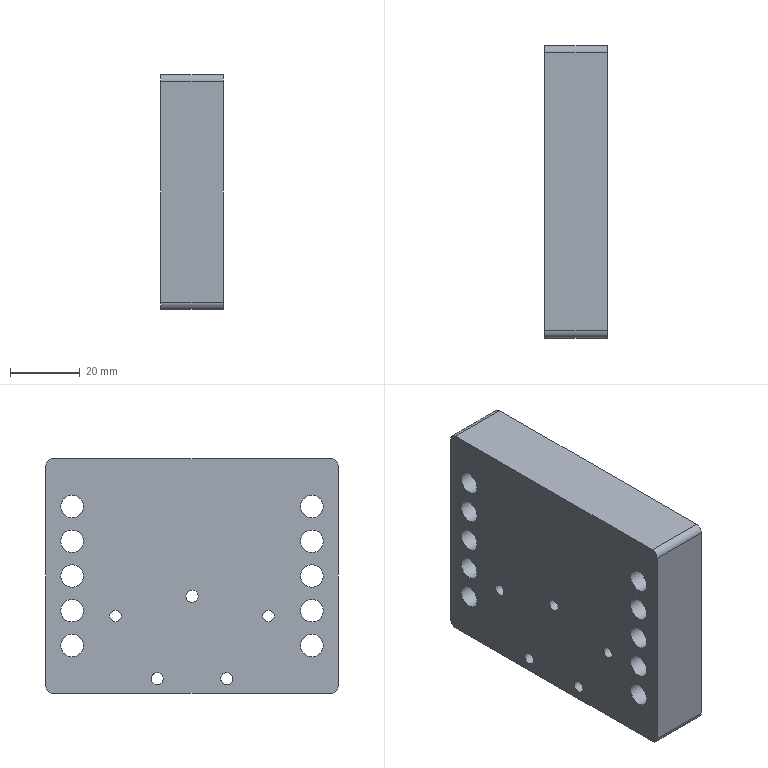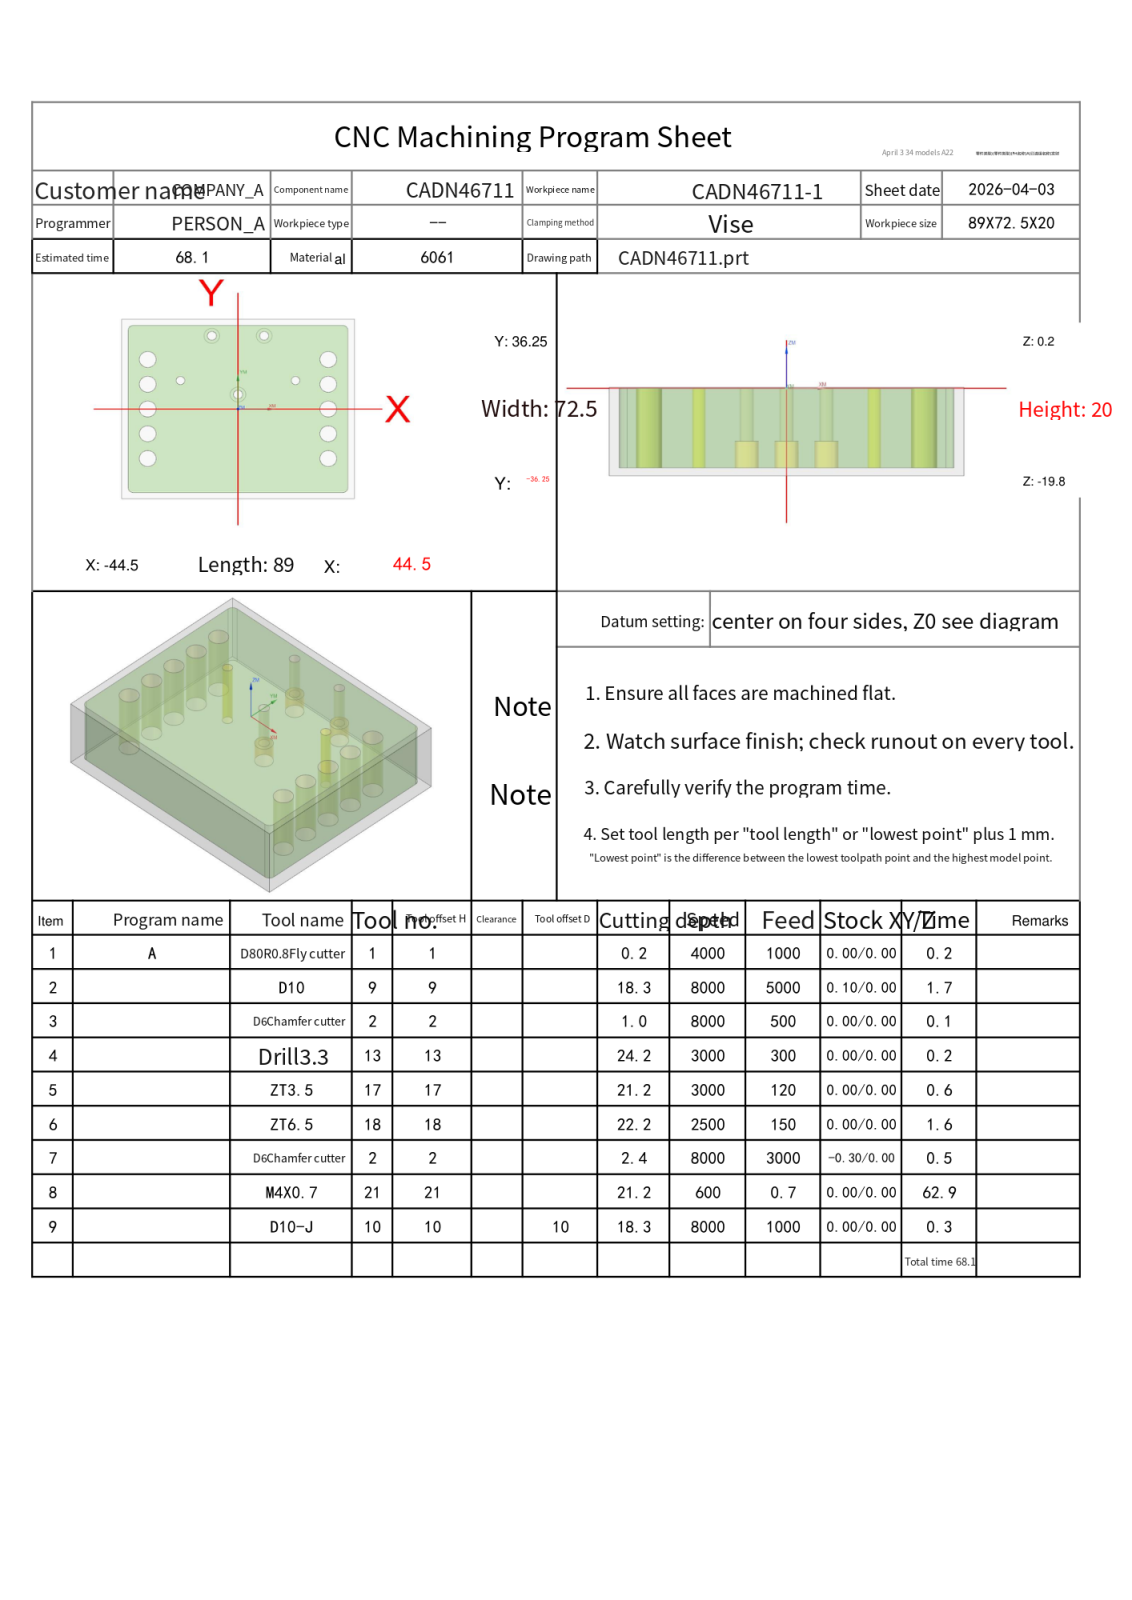NC program | NX | posted by the shop | part box 18 x 84 x 67.5 mm
Whole program:
%
O0001
(Machine time: 129.73 MIN)
(===Total Tool:8===)
(T1=D80R0.8 Fly cutter D=80.  R=0.8  D-  H01 Z=-0.   )
(T9=D10     D=10.  R=0.   D-  H09 Z=-18.1 )
(T2=D6 Chamfer cutter   D=6.   R=0.   D-  H02 Z=-2.2  )
(T13=Drill 3.3  D=3.3  DR_a=118 D-  H13 Z=-23.99)
(T17=ZT3.5  D=3.5  DR_a=118 D-  H17 Z=-21.  )
(T18=ZT6.5  D=6.5  DR_a=118 D-  H18 Z=-21.95)
(T21=M4X0.7 D=3.3  DR_a=180 D-  H21 Z=-21.  )
(T10=D10-J  D=10.  R=0.   D10 H10 Z=-18.1 )
G80 G90 G17 G49 G40
G91 G28 Z0
M01
N1 T01 M06
(D80R0.8 Fly cutter  D=80. R=0.8 H=01 ce=0.00 di=0.00)
G00 G90 G54 X-87. Y0.0 M03 S4000
G43 H01 Z20.
M08
Z2.
G01 Z0.0 F1000.
X-82.
X82.
X87.
Z2.
G00 Z20.
G91 G28 Z0.0
M05
M09
G91 G28 Z0.0
M01
N2 T09 M06
(D10  D=10. R=0. H=09 ce=0.10 di=0.00)
G00 G90 G54 X0.0 Y-38.85 M03 S8000
G43 H09 Z20.
M08
Z.5
G01 X-40. Z.407 F5000.
G02 X-47.1 Y-31.75 Z.38 I0.0 J7.1
G01 Y31.75 Z.232
G02 X-40. Y38.85 Z.206 I7.1 J0.0
G01 X40. Z.019
G02 X47.1 Y31.75 Z-.007 I0.0 J-7.1
G01 Y-31.75 Z-.155
G02 X40. Y-38.85 Z-.182 I-7.1 J0.0
G01 X-40. Z-.368
G02 X-47.1 Y-31.75 Z-.395 I0.0 J7.1
G01 Y31.75 Z-.543
G02 X-40. Y38.85 Z-.569 I7.1 J0.0
G01 X40. Z-.756
G02 X47.1 Y31.75 Z-.782 I0.0 J-7.1
G01 Y-31.75 Z-.93
G02 X40. Y-38.85 Z-.957 I-7.1 J0.0
G01 X-40. Z-1.143
G02 X-47.1 Y-31.75 Z-1.17 I0.0 J7.1
G01 Y31.75 Z-1.318
G02 X-40. Y38.85 Z-1.344 I7.1 J0.0
G01 X40. Z-1.531
G02 X47.1 Y31.75 Z-1.557 I0.0 J-7.1
G01 Y-31.75 Z-1.705
G02 X40. Y-38.85 Z-1.732 I-7.1 J0.0
G01 X-40. Z-1.918
G02 X-47.1 Y-31.75 Z-1.945 I0.0 J7.1
G01 Y31.75 Z-2.093
G02 X-40. Y38.85 Z-2.119 I7.1 J0.0
G01 X40. Z-2.306
G02 X47.1 Y31.75 Z-2.332 I0.0 J-7.1
G01 Y-31.75 Z-2.48
G02 X40. Y-38.85 Z-2.507 I-7.1 J0.0
G01 X-40. Z-2.693
G02 X-47.1 Y-31.75 Z-2.72 I0.0 J7.1
G01 Y31.75 Z-2.868
G02 X-40. Y38.85 Z-2.894 I7.1 J0.0
G01 X40. Z-3.081
G02 X47.1 Y31.75 Z-3.107 I0.0 J-7.1
G01 Y-31.75 Z-3.255
G02 X40. Y-38.85 Z-3.282 I-7.1 J0.0
G01 X-40. Z-3.468
G02 X-47.1 Y-31.75 Z-3.495 I0.0 J7.1
G01 Y31.75 Z-3.643
G02 X-40. Y38.85 Z-3.669 I7.1 J0.0
G01 X40. Z-3.856
G02 X47.1 Y31.75 Z-3.882 I0.0 J-7.1
G01 Y-31.75 Z-4.03
G02 X40. Y-38.85 Z-4.057 I-7.1 J0.0
G01 X-40. Z-4.243
G02 X-47.1 Y-31.75 Z-4.27 I0.0 J7.1
G01 Y31.75 Z-4.418
G02 X-40. Y38.85 Z-4.444 I7.1 J0.0
G01 X40. Z-4.631
G02 X47.1 Y31.75 Z-4.657 I0.0 J-7.1
G01 Y-31.75 Z-4.805
G02 X40. Y-38.85 Z-4.832 I-7.1 J0.0
G01 X-40. Z-5.018
G02 X-47.1 Y-31.75 Z-5.045 I0.0 J7.1
G01 Y31.75 Z-5.193
G02 X-40. Y38.85 Z-5.219 I7.1 J0.0
G01 X40. Z-5.406
G02 X47.1 Y31.75 Z-5.432 I0.0 J-7.1
G01 Y-31.75 Z-5.58
G02 X40. Y-38.85 Z-5.607 I-7.1 J0.0
G01 X-40. Z-5.793
G02 X-47.1 Y-31.75 Z-5.82 I0.0 J7.1
G01 Y31.75 Z-5.968
G02 X-40. Y38.85 Z-5.994 I7.1 J0.0
G01 X40. Z-6.181
G02 X47.1 Y31.75 Z-6.207 I0.0 J-7.1
G01 Y-31.75 Z-6.355
G02 X40. Y-38.85 Z-6.382 I-7.1 J0.0
G01 X-40. Z-6.568
G02 X-47.1 Y-31.75 Z-6.595 I0.0 J7.1
G01 Y31.75 Z-6.743
G02 X-40. Y38.85 Z-6.769 I7.1 J0.0
G01 X40. Z-6.956
G02 X47.1 Y31.75 Z-6.982 I0.0 J-7.1
G01 Y-31.75 Z-7.13
G02 X40. Y-38.85 Z-7.157 I-7.1 J0.0
G01 X-40. Z-7.343
G02 X-47.1 Y-31.75 Z-7.37 I0.0 J7.1
G01 Y31.75 Z-7.518
G02 X-40. Y38.85 Z-7.544 I7.1 J0.0
G01 X40. Z-7.731
G02 X47.1 Y31.75 Z-7.757 I0.0 J-7.1
G01 Y-31.75 Z-7.905
G02 X40. Y-38.85 Z-7.932 I-7.1 J0.0
G01 X-40. Z-8.118
G02 X-47.1 Y-31.75 Z-8.145 I0.0 J7.1
G01 Y31.75 Z-8.293
G02 X-40. Y38.85 Z-8.319 I7.1 J0.0
G01 X40. Z-8.506
G02 X47.1 Y31.75 Z-8.532 I0.0 J-7.1
G01 Y-31.75 Z-8.68
G02 X40. Y-38.85 Z-8.707 I-7.1 J0.0
G01 X-40. Z-8.893
G02 X-47.1 Y-31.75 Z-8.92 I0.0 J7.1
G01 Y31.75 Z-9.068
G02 X-40. Y38.85 Z-9.094 I7.1 J0.0
G01 X40. Z-9.281
G02 X47.1 Y31.75 Z-9.307 I0.0 J-7.1
G01 Y-31.75 Z-9.455
G02 X40. Y-38.85 Z-9.482 I-7.1 J0.0
G01 X-40. Z-9.668
G02 X-47.1 Y-31.75 Z-9.695 I0.0 J7.1
G01 Y31.75 Z-9.843
G02 X-40. Y38.85 Z-9.869 I7.1 J0.0
G01 X40. Z-10.056
G02 X47.1 Y31.75 Z-10.082 I0.0 J-7.1
G01 Y-31.75 Z-10.23
G02 X40. Y-38.85 Z-10.257 I-7.1 J0.0
G01 X-40. Z-10.443
G02 X-47.1 Y-31.75 Z-10.47 I0.0 J7.1
G01 Y31.75 Z-10.618
G02 X-40. Y38.85 Z-10.644 I7.1 J0.0
G01 X40. Z-10.831
G02 X47.1 Y31.75 Z-10.857 I0.0 J-7.1
G01 Y-31.75 Z-11.005
G02 X40. Y-38.85 Z-11.032 I-7.1 J0.0
G01 X-40. Z-11.218
G02 X-47.1 Y-31.75 Z-11.245 I0.0 J7.1
G01 Y31.75 Z-11.393
G02 X-40. Y38.85 Z-11.419 I7.1 J0.0
G01 X40. Z-11.606
G02 X47.1 Y31.75 Z-11.632 I0.0 J-7.1
G01 Y-31.75 Z-11.78
G02 X40. Y-38.85 Z-11.807 I-7.1 J0.0
G01 X-40. Z-11.993
G02 X-47.1 Y-31.75 Z-12.02 I0.0 J7.1
G01 Y31.75 Z-12.168
G02 X-40. Y38.85 Z-12.194 I7.1 J0.0
G01 X40. Z-12.381
G02 X47.1 Y31.75 Z-12.407 I0.0 J-7.1
G01 Y-31.75 Z-12.555
G02 X40. Y-38.85 Z-12.582 I-7.1 J0.0
G01 X-40. Z-12.768
G02 X-47.1 Y-31.75 Z-12.795 I0.0 J7.1
G01 Y31.75 Z-12.943
G02 X-40. Y38.85 Z-12.969 I7.1 J0.0
G01 X40. Z-13.156
G02 X47.1 Y31.75 Z-13.182 I0.0 J-7.1
G01 Y-31.75 Z-13.33
G02 X40. Y-38.85 Z-13.357 I-7.1 J0.0
G01 X-40. Z-13.543
G02 X-47.1 Y-31.75 Z-13.57 I0.0 J7.1
G01 Y31.75 Z-13.718
G02 X-40. Y38.85 Z-13.744 I7.1 J0.0
G01 X40. Z-13.931
G02 X47.1 Y31.75 Z-13.957 I0.0 J-7.1
G01 Y-31.75 Z-14.105
G02 X40. Y-38.85 Z-14.132 I-7.1 J0.0
G01 X-40. Z-14.318
G02 X-47.1 Y-31.75 Z-14.345 I0.0 J7.1
G01 Y31.75 Z-14.493
G02 X-40. Y38.85 Z-14.519 I7.1 J0.0
G01 X40. Z-14.706
G02 X47.1 Y31.75 Z-14.732 I0.0 J-7.1
G01 Y-31.75 Z-14.88
G02 X40. Y-38.85 Z-14.907 I-7.1 J0.0
G01 X-40. Z-15.093
G02 X-47.1 Y-31.75 Z-15.12 I0.0 J7.1
G01 Y31.75 Z-15.268
G02 X-40. Y38.85 Z-15.294 I7.1 J0.0
G01 X40. Z-15.481
G02 X47.1 Y31.75 Z-15.507 I0.0 J-7.1
G01 Y-31.75 Z-15.655
G02 X40. Y-38.85 Z-15.682 I-7.1 J0.0
G01 X-40. Z-15.868
G02 X-47.1 Y-31.75 Z-15.895 I0.0 J7.1
G01 Y31.75 Z-16.043
G02 X-40. Y38.85 Z-16.069 I7.1 J0.0
G01 X40. Z-16.256
G02 X47.1 Y31.75 Z-16.282 I0.0 J-7.1
G01 Y-31.75 Z-16.43
G02 X40. Y-38.85 Z-16.457 I-7.1 J0.0
G01 X-40. Z-16.643
G02 X-47.1 Y-31.75 Z-16.67 I0.0 J7.1
G01 Y31.75 Z-16.818
G02 X-40. Y38.85 Z-16.844 I7.1 J0.0
G01 X40. Z-17.031
G02 X47.1 Y31.75 Z-17.057 I0.0 J-7.1
G01 Y-31.75 Z-17.205
G02 X40. Y-38.85 Z-17.232 I-7.1 J0.0
G01 X-40. Z-17.418
G02 X-47.1 Y-31.75 Z-17.445 I0.0 J7.1
G01 Y31.75 Z-17.593
G02 X-40. Y38.85 Z-17.619 I7.1 J0.0
G01 X40. Z-17.806
G02 X47.1 Y31.75 Z-17.832 I0.0 J-7.1
G01 Y-31.75 Z-17.98
G02 X40. Y-38.85 Z-18.007 I-7.1 J0.0
G01 X0.0 Z-18.1
X-40.
G02 X-47.1 Y-31.75 I0.0 J7.1
G01 Y31.75
G02 X-40. Y38.85 I7.1 J0.0
G01 X40.
G02 X47.1 Y31.75 I0.0 J-7.1
G01 Y-31.75
G02 X40. Y-38.85 I-7.1 J0.0
G01 X0.0
X-.5
Z-17.1
G00 Z20.
G91 G28 Z0.0
M05
M09
G91 G28 Z0.0
M01
N3 T02 M06
(D6 Chamfer cutter  D=6. R=0. H=02 ce=0.00 di=0.00)
G00 G90 G54 X-34.5 Y-20. M03 S8000
G43 H02 Z20.
M08
G98 G81 X-34.5 Y-20. Z-.8 R1. F500.
Y-10.
Y0.0
Y10.
Y20.
X-22. Y11.5
X-10. Y29.55
X10.
X0.0 Y5.85
X22. Y11.5
X34.5 Y20.
Y10.
Y0.0
Y-10.
Y-20.
G80
G00 Z20.
G91 G28 Z0.0
M05
M09
G91 G28 Z0.0
M01
N4 T13 M06
(Drill 3.3 D=3.3 DR_a=118 H=13)
G00 G90 G54 X-22. Y11.5 M03 S3000
G43 H13 Z20.
M08
G98 G83 X-22. Y11.5 Z-23.991 R1. F300. Q2.
X22.
G80
G00 Z20.
G91 G28 Z0.0
M05
M09
G91 G28 Z0.0
M01
N5 T17 M06
(ZT3.5 D=3.5 DR_a=118 H=17)
G00 G90 G54 X-10. Y29.55 M03 S3000
G43 H17 Z20.
M08
G98 G83 X-10. Y29.55 Z-21. R1. F120. Q3.
X10.
X0.0 Y5.85
G80
G00 Z20.
G91 G28 Z0.0
M05
M09
G91 G28 Z0.0
M01
N6 T18 M06
(ZT6.5 D=6.5 DR_a=118 H=18)
G00 G90 G54 X34.5 Y-20. M03 S2500
G43 H18 Z20.
M08
G98 G83 X34.5 Y-20. Z-21.953 R1. F150. Q3.
Y-10.
Y0.0
Y10.
Y20.
X-34.5
Y10.
Y0.0
Y-10.
Y-20.
G80
G00 Z20.
G91 G28 Z0.0
M05
M09
G91 G28 Z0.0
M01
N7 T02 M06
(D6 Chamfer cutter  D=6. R=0. H=02 ce=0.00 di=0.00)
G00 G90 G54 X-.25 Y35.578 M03 S8000
G43 H02 Z20.
M08
Z2.399
G01 Z-1.5 F3000.
G03 X-.33 Y35.278 I.52 J-.3
X-.03 Y34.758 I.6 J0.0
G01 X0.0 Y34.75
X40.
G02 X43. Y31.75 I0.0 J-3.
G01 Y-31.75
G02 X40. Y-34.75 I-3. J0.0
G01 X-40.
G02 X-43. Y-31.75 I0.0 J3.
G01 Y31.75
G02 X-40. Y34.75 I3. J0.0
G01 X0.0
X.03 Y34.758
G03 X.33 Y35.278 I-.3 J.52
X.25 Y35.578 I-.6 J0.0
G01 Z2.399
G00 Z20.
G00 G90 X-22. Y11.5 M03 S8000
Z20.
G98 G81 X-22. Y11.5 Z-2.2 R3. F500.
X22.
G80
G00 Z20.
G00 G90 X-10. Y29.55 M03 S8000
Z20.
G98 G81 X-10. Y29.55 Z-2.05 R3. F500.
X10.
X0.0 Y5.85
G80
G00 Z20.
G00 G90 X-36. Y19.609 M03 S8000
Z20.
Z-.5
G01 Z-1. F800.
Y18.95
G03 X-34.5 Y17.45 I1.5 J0.0
X-31.95 Y20. I0.0 J2.55
X-34.5 Y22.55 I-2.55 J0.0
X-37.05 Y20. I0.0 J-2.55
X-34.5 Y17.45 I2.55 J0.0
X-33. Y18.95 I0.0 J1.5
G01 Y19.609
Z-.5
G00 Z20.
X-36. Y9.609
Z-.5
G01 Z-1.
Y8.95
G03 X-34.5 Y7.45 I1.5 J0.0
X-31.95 Y10. I0.0 J2.55
X-34.5 Y12.55 I-2.55 J0.0
X-37.05 Y10. I0.0 J-2.55
X-34.5 Y7.45 I2.55 J0.0
X-33. Y8.95 I0.0 J1.5
G01 Y9.609
Z-.5
G00 Z20.
X-36. Y-.391
Z-.5
G01 Z-1.
Y-1.05
G03 X-34.5 Y-2.55 I1.5 J0.0
X-31.95 Y0.0 I0.0 J2.55
X-34.5 Y2.55 I-2.55 J0.0
X-37.05 Y0.0 I0.0 J-2.55
X-34.5 Y-2.55 I2.55 J0.0
X-33. Y-1.05 I0.0 J1.5
G01 Y-.391
Z-.5
G00 Z20.
X-36. Y-10.391
Z-.5
G01 Z-1.
Y-11.05
G03 X-34.5 Y-12.55 I1.5 J0.0
X-31.95 Y-10. I0.0 J2.55
X-34.5 Y-7.45 I-2.55 J0.0
X-37.05 Y-10. I0.0 J-2.55
X-34.5 Y-12.55 I2.55 J0.0
X-33. Y-11.05 I0.0 J1.5
G01 Y-10.391
Z-.5
G00 Z20.
X-36. Y-20.391
Z-.5
G01 Z-1.
Y-21.05
G03 X-34.5 Y-22.55 I1.5 J0.0
X-31.95 Y-20. I0.0 J2.55
X-34.5 Y-17.45 I-2.55 J0.0
X-37.05 Y-20. I0.0 J-2.55
X-34.5 Y-22.55 I2.55 J0.0
X-33. Y-21.05 I0.0 J1.5
G01 Y-20.391
Z-.5
G00 Z20.
X33.
Z-.5
G01 Z-1.
Y-21.05
G03 X34.5 Y-22.55 I1.5 J0.0
X37.05 Y-20. I0.0 J2.55
X34.5 Y-17.45 I-2.55 J0.0
X31.95 Y-20. I0.0 J-2.55
X34.5 Y-22.55 I2.55 J0.0
X36. Y-21.05 I0.0 J1.5
G01 Y-20.391
Z-.5
G00 Z20.
X33. Y-10.391
Z-.5
G01 Z-1.
Y-11.05
G03 X34.5 Y-12.55 I1.5 J0.0
X37.05 Y-10. I0.0 J2.55
X34.5 Y-7.45 I-2.55 J0.0
X31.95 Y-10. I0.0 J-2.55
X34.5 Y-12.55 I2.55 J0.0
X36. Y-11.05 I0.0 J1.5
G01 Y-10.391
Z-.5
G00 Z20.
X33. Y-.391
Z-.5
G01 Z-1.
Y-1.05
G03 X34.5 Y-2.55 I1.5 J0.0
X37.05 Y0.0 I0.0 J2.55
X34.5 Y2.55 I-2.55 J0.0
X31.95 Y0.0 I0.0 J-2.55
X34.5 Y-2.55 I2.55 J0.0
X36. Y-1.05 I0.0 J1.5
G01 Y-.391
Z-.5
G00 Z20.
X33. Y9.609
Z-.5
G01 Z-1.
Y8.95
G03 X34.5 Y7.45 I1.5 J0.0
X37.05 Y10. I0.0 J2.55
X34.5 Y12.55 I-2.55 J0.0
X31.95 Y10. I0.0 J-2.55
X34.5 Y7.45 I2.55 J0.0
X36. Y8.95 I0.0 J1.5
G01 Y9.609
Z-.5
G00 Z20.
X33. Y19.609
Z-.5
G01 Z-1.
Y18.95
G03 X34.5 Y17.45 I1.5 J0.0
X37.05 Y20. I0.0 J2.55
X34.5 Y22.55 I-2.55 J0.0
X31.95 Y20. I0.0 J-2.55
X34.5 Y17.45 I2.55 J0.0
X36. Y18.95 I0.0 J1.5
G01 Y19.609
Z-.5
G00 Z20.
G91 G28 Z0.0
M05
M09
G91 G28 Z0.0
M01
N8 T21 M06
(M4X0.7 D=3.3 DR_a=180 H=21)
G00 G90 G54 X-22. Y11.5 M03 S600
G43 H21 Z20.
M08
G95
G98 G84 X-22. Y11.5 Z-21. R1. F.7 Q4.
X22.
G80
G94
G00 Z20.
G91 G28 Z0.0
M05
M09
G91 G28 Z0.0
M01
N9 T10 M06
(D10-J  D=10. R=0. H=10 ce=0.00 di=0.00)
G00 G90 G54 X41.011 Y-39.887 M03 S8000
G43 H10 Z20.
M08
Z-17.6
G01 Z-18.1 F1000.
G41 D10
X40.998 Y-39.688
G03 X40. Y-38.75 I-.998 J-.063
G01 X-40.
G02 X-47. Y-31.75 I0.0 J7.
G01 Y31.75
G02 X-40. Y38.75 I7. J0.0
G01 X40.
G02 X47. Y31.75 I0.0 J-7.
G01 Y-31.75
G02 X40. Y-38.75 I-7. J0.0
G01 X39.5
G03 X38.5 Y-39.75 I0.0 J-1.
G01 G40 Y-39.95
Z-17.6
G00 Z20.
M05
M09
G91 G28 Z0.0
G91 G28 Y0.0
M30
%